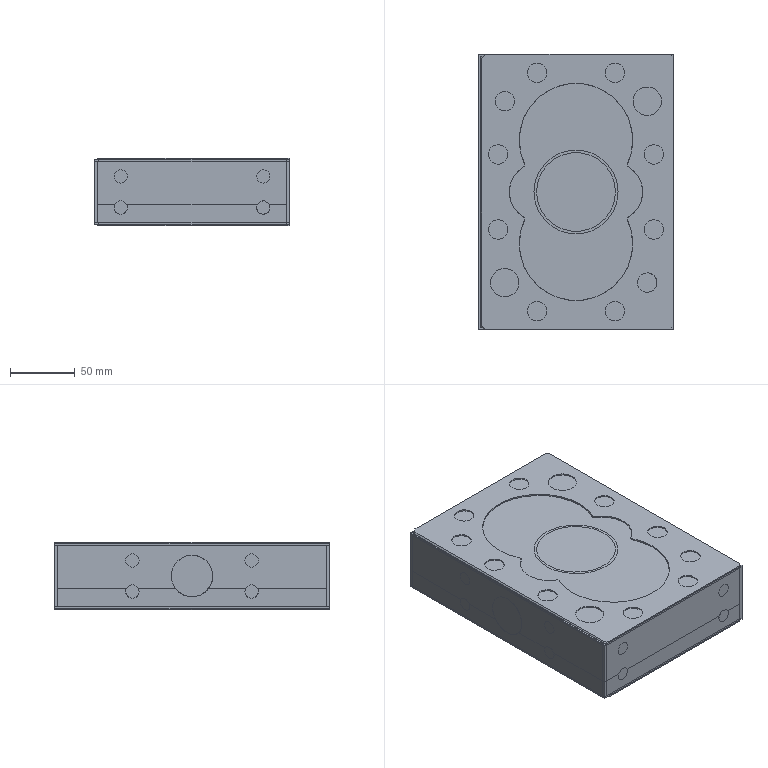NC program | NX | posted with a generic post | part box 150.2 x 212.2 x 52.4 mm
Lines 18 to 851 of 152230:
(PLANAR_PROFILE , TOOL : D45R0.8圆鼻飞刀)
N34 T06 M6
N36 G54
N38 G17 G0 G90 X-44.794 Y20.59 S1061 M3
N40 G43 Z100. H6
N42 Z1.1
N44 G94 G1 X-47.122 Y19.947 Z1.096 F1273.
N46 X-49.964 Y18.69 Z1.09
N48 X-52.591 Y17.031 Z1.085
N50 X-54.947 Y15.006 Z1.08
N52 X-56.982 Y12.658 Z1.074
N54 X-58.651 Y10.037 Z1.069
N56 X-59.918 Y7.201 Z1.063
N58 X-60.758 Y4.209 Z1.058
N60 X-61.15 Y1.127 Z1.052
N62 Y-1.127 Z1.048
N64 X-60.758 Y-4.209 Z1.043
N66 X-59.918 Y-7.201 Z1.038
N68 X-58.651 Y-10.037 Z1.032
N70 X-56.982 Y-12.658 Z1.027
N72 X-54.947 Y-15.006 Z1.021
N74 X-52.591 Y-17.031 Z1.016
N76 X-49.964 Y-18.69 Z1.011
N78 X-47.122 Y-19.947 Z1.005
N80 X-44.127 Y-20.774 Z1.
N82 X-41.043 Y-21.154 Z0.994
N84 X-37.937 Y-21.079 Z0.989
N86 X-34.876 Y-20.551 Z0.983
N88 X-31.924 Y-19.58 Z0.978
N90 X-29.855 Y-18.595 Z0.974
N92 X-27.425 Y-17.746 Z0.969
N94 X-24.914 Y-17.178 Z0.965
N96 X-22.355 Y-16.9 Z0.96
N98 X-18.735 Z0.954
N100 X-15.612 Y-17.28 Z0.949
N102 X-12.572 Y-18.089 Z0.943
N104 X-9.673 Y-19.313 Z0.938
N106 X-6.972 Y-20.926 Z0.932
N108 X-4.521 Y-22.899 Z0.927
N110 X-2.367 Y-25.192 Z0.921
N112 X-0.552 Y-27.762 Z0.916
N114 X0. Y-28.787 Z0.914
N116 X0.552 Y-27.762 Z0.912
N118 X2.367 Y-25.192 Z0.906
N120 X4.521 Y-22.899 Z0.901
N122 X6.972 Y-20.926 Z0.895
N124 X9.673 Y-19.313 Z0.89
N126 X12.572 Y-18.089 Z0.884
N128 X15.612 Y-17.28 Z0.879
N130 X18.735 Y-16.9 Z0.873
N132 X22.355 Z0.867
N134 X24.914 Y-17.178 Z0.862
N136 X27.425 Y-17.746 Z0.858
N138 X29.855 Y-18.595 Z0.853
N140 X31.924 Y-19.58 Z0.849
N142 X34.876 Y-20.551 Z0.844
N144 X37.937 Y-21.079 Z0.839
N146 X41.043 Y-21.154 Z0.833
N148 X44.127 Y-20.774 Z0.828
N150 X47.122 Y-19.947 Z0.822
N152 X49.964 Y-18.69 Z0.817
N154 X52.591 Y-17.031 Z0.811
N156 X54.947 Y-15.006 Z0.806
N158 X56.982 Y-12.658 Z0.801
N160 X58.651 Y-10.037 Z0.795
N162 X59.918 Y-7.201 Z0.79
N164 X60.758 Y-4.209 Z0.784
N166 X61.15 Y-1.127 Z0.779
N168 Y0. Z0.777
N170 Y1.127 Z0.775
N172 X60.758 Y4.209 Z0.77
N174 X59.918 Y7.201 Z0.764
N176 X58.651 Y10.037 Z0.759
N178 X56.982 Y12.658 Z0.753
N180 X54.947 Y15.006 Z0.748
N182 X52.591 Y17.031 Z0.742
N184 X49.964 Y18.69 Z0.737
N186 X47.122 Y19.947 Z0.732
N188 X44.127 Y20.774 Z0.726
N190 X41.043 Y21.154 Z0.721
N192 X37.937 Y21.079 Z0.715
N194 X34.876 Y20.551 Z0.71
N196 X31.924 Y19.58 Z0.705
N198 X29.855 Y18.595 Z0.701
N200 X27.425 Y17.746 Z0.696
N202 X24.914 Y17.178 Z0.692
N204 X22.355 Y16.9 Z0.687
N206 X18.735 Z0.681
N208 X15.612 Y17.28 Z0.675
N210 X12.572 Y18.089 Z0.67
N212 X9.673 Y19.313 Z0.664
N214 X6.972 Y20.926 Z0.659
N216 X4.521 Y22.899 Z0.653
N218 X2.367 Y25.192 Z0.648
N220 X0.552 Y27.762 Z0.642
N222 X0. Y28.787 Z0.64
N224 X-0.552 Y27.762 Z0.638
N226 X-2.367 Y25.192 Z0.633
N228 X-4.521 Y22.899 Z0.627
N230 X-6.972 Y20.926 Z0.622
N232 X-9.673 Y19.313 Z0.616
N234 X-12.572 Y18.089 Z0.611
N236 X-15.612 Y17.28 Z0.605
N238 X-18.735 Y16.9 Z0.6
N240 X-22.355 Z0.593
N242 X-24.914 Y17.178 Z0.589
N244 X-27.425 Y17.746 Z0.584
N246 X-29.855 Y18.595 Z0.58
N248 X-31.924 Y19.58 Z0.576
N250 X-34.876 Y20.551 Z0.571
N252 X-37.937 Y21.079 Z0.565
N254 X-41.043 Y21.154 Z0.56
N256 X-44.127 Y20.774 Z0.554
N258 X-47.122 Y19.947 Z0.549
N260 X-49.964 Y18.69 Z0.543
N262 X-52.591 Y17.031 Z0.538
N264 X-54.947 Y15.006 Z0.533
N266 X-56.982 Y12.658 Z0.527
N268 X-58.651 Y10.037 Z0.522
N270 X-59.918 Y7.201 Z0.516
N272 X-60.758 Y4.209 Z0.511
N274 X-61.15 Y1.127 Z0.505
N276 Y-1.127 Z0.502
N278 X-60.758 Y-4.209 Z0.496
N280 X-59.918 Y-7.201 Z0.491
N282 X-58.651 Y-10.037 Z0.485
N284 X-56.982 Y-12.658 Z0.48
N286 X-54.947 Y-15.006 Z0.474
N288 X-52.591 Y-17.031 Z0.469
N290 X-49.964 Y-18.69 Z0.464
N292 X-47.122 Y-19.947 Z0.458
N294 X-44.127 Y-20.774 Z0.453
N296 X-41.043 Y-21.154 Z0.447
N298 X-37.937 Y-21.079 Z0.442
N300 X-34.876 Y-20.551 Z0.436
N302 X-31.924 Y-19.58 Z0.431
N304 X-29.855 Y-18.595 Z0.427
N306 X-27.425 Y-17.746 Z0.423
N308 X-24.914 Y-17.178 Z0.418
N310 X-22.355 Y-16.9 Z0.414
N312 X-18.735 Z0.407
N314 X-15.612 Y-17.28 Z0.402
N316 X-12.572 Y-18.089 Z0.396
N318 X-9.673 Y-19.313 Z0.391
N320 X-6.972 Y-20.926 Z0.385
N322 X-4.521 Y-22.899 Z0.38
N324 X-2.367 Y-25.192 Z0.374
N326 X-0.552 Y-27.762 Z0.369
N328 X0. Y-28.787 Z0.367
N330 X0.552 Y-27.762 Z0.365
N332 X2.367 Y-25.192 Z0.359
N334 X4.521 Y-22.899 Z0.354
N336 X6.972 Y-20.926 Z0.348
N338 X9.673 Y-19.313 Z0.343
N340 X12.572 Y-18.089 Z0.337
N342 X15.612 Y-17.28 Z0.332
N344 X18.735 Y-16.9 Z0.326
N346 X22.355 Z0.32
N348 X24.914 Y-17.178 Z0.316
N350 X27.425 Y-17.746 Z0.311
N352 X29.855 Y-18.595 Z0.307
N354 X31.924 Y-19.58 Z0.303
N356 X34.876 Y-20.551 Z0.297
N358 X37.937 Y-21.079 Z0.292
N360 X41.043 Y-21.154 Z0.286
N362 X44.127 Y-20.774 Z0.281
N364 X47.122 Y-19.947 Z0.275
N366 X49.964 Y-18.69 Z0.27
N368 X52.591 Y-17.031 Z0.265
N370 X54.947 Y-15.006 Z0.259
N372 X56.982 Y-12.658 Z0.254
N374 X58.651 Y-10.037 Z0.248
N376 X59.918 Y-7.201 Z0.243
N378 X60.758 Y-4.209 Z0.237
N380 X61.15 Y-1.127 Z0.232
N382 Y0. Z0.23
N384 Y1.127 Z0.228
N386 X60.758 Y4.209 Z0.223
N388 X59.918 Y7.201 Z0.217
N390 X58.651 Y10.037 Z0.212
N392 X56.982 Y12.658 Z0.206
N394 X54.947 Y15.006 Z0.201
N396 X52.591 Y17.031 Z0.196
N398 X49.964 Y18.69 Z0.19
N400 X47.122 Y19.947 Z0.185
N402 X44.127 Y20.774 Z0.179
N404 X41.043 Y21.154 Z0.174
N406 X37.937 Y21.079 Z0.168
N408 X34.876 Y20.551 Z0.163
N410 X31.924 Y19.58 Z0.158
N412 X29.855 Y18.595 Z0.154
N414 X27.425 Y17.746 Z0.149
N416 X24.914 Y17.178 Z0.145
N418 X22.355 Y16.9 Z0.14
N420 X18.735 Z0.134
N422 X15.612 Y17.28 Z0.128
N424 X12.572 Y18.089 Z0.123
N426 X9.673 Y19.313 Z0.117
N428 X6.972 Y20.926 Z0.112
N430 X4.521 Y22.899 Z0.106
N432 X2.367 Y25.192 Z0.101
N434 X0.552 Y27.762 Z0.095
N436 X0. Y28.787 Z0.093
N438 X-0.552 Y27.762 Z0.091
N440 X-2.367 Y25.192 Z0.086
N442 X-4.521 Y22.899 Z0.08
N444 X-6.972 Y20.926 Z0.075
N446 X-9.673 Y19.313 Z0.069
N448 X-12.572 Y18.089 Z0.064
N450 X-15.612 Y17.28 Z0.058
N452 X-18.735 Y16.9 Z0.053
N454 X-22.355 Z0.047
N456 X-24.914 Y17.178 Z0.042
N458 X-27.425 Y17.746 Z0.038
N460 X-29.855 Y18.595 Z0.033
N462 X-31.924 Y19.58 Z0.029
N464 X-34.876 Y20.551 Z0.024
N466 X-37.937 Y21.079 Z0.018
N468 X-41.043 Y21.154 Z0.013
N470 X-44.127 Y20.774 Z0.007
N472 X-47.122 Y19.947 Z0.002
N474 X-49.964 Y18.69 Z-0.003
N476 X-52.591 Y17.031 Z-0.009
N478 X-54.947 Y15.006 Z-0.014
N480 X-56.982 Y12.658 Z-0.02
N482 X-58.651 Y10.037 Z-0.025
N484 X-59.918 Y7.201 Z-0.031
N486 X-60.758 Y4.209 Z-0.036
N488 X-61.15 Y1.127 Z-0.041
N490 Y-1.127 Z-0.045
N492 X-60.758 Y-4.209 Z-0.051
N494 X-59.918 Y-7.201 Z-0.056
N496 X-58.651 Y-10.037 Z-0.062
N498 X-56.982 Y-12.658 Z-0.067
N500 X-54.947 Y-15.006 Z-0.072
N502 X-52.591 Y-17.031 Z-0.078
N504 X-49.964 Y-18.69 Z-0.083
N506 X-47.122 Y-19.947 Z-0.089
N508 X-44.127 Y-20.774 Z-0.094
N510 X-41.043 Y-21.154 Z-0.1
N512 X-37.937 Y-21.079 Z-0.105
N514 X-34.876 Y-20.551 Z-0.11
N516 X-31.924 Y-19.58 Z-0.116
N518 X-29.855 Y-18.595 Z-0.12
N520 X-27.425 Y-17.746 Z-0.124
N522 X-24.914 Y-17.178 Z-0.129
N524 X-22.355 Y-16.9 Z-0.133
N526 X-18.735 Z-0.14
N528 X-15.612 Y-17.28 Z-0.145
N530 X-12.572 Y-18.089 Z-0.151
N532 X-9.673 Y-19.313 Z-0.156
N534 X-6.972 Y-20.926 Z-0.162
N536 X-4.521 Y-22.899 Z-0.167
N538 X-2.367 Y-25.192 Z-0.173
N540 X-0.552 Y-27.762 Z-0.178
N542 X0. Y-28.787 Z-0.18
N544 X0.552 Y-27.762 Z-0.182
N546 X2.367 Y-25.192 Z-0.188
N548 X4.521 Y-22.899 Z-0.193
N550 X6.972 Y-20.926 Z-0.199
N552 X9.673 Y-19.313 Z-0.204
N554 X12.572 Y-18.089 Z-0.21
N556 X15.612 Y-17.28 Z-0.215
N558 X18.735 Y-16.9 Z-0.221
N560 X22.355 Z-0.227
N562 X24.914 Y-17.178 Z-0.231
N564 X27.425 Y-17.746 Z-0.236
N566 X29.855 Y-18.595 Z-0.24
N568 X31.924 Y-19.58 Z-0.244
N570 X34.876 Y-20.551 Z-0.25
N572 X37.937 Y-21.079 Z-0.255
N574 X41.043 Y-21.154 Z-0.261
N576 X44.127 Y-20.774 Z-0.266
N578 X47.122 Y-19.947 Z-0.272
N580 X49.964 Y-18.69 Z-0.277
N582 X52.591 Y-17.031 Z-0.282
N584 X54.947 Y-15.006 Z-0.288
N586 X56.982 Y-12.658 Z-0.293
N588 X58.651 Y-10.037 Z-0.299
N590 X59.918 Y-7.201 Z-0.304
N592 X60.758 Y-4.209 Z-0.309
N594 X61.15 Y-1.127 Z-0.315
N596 Y0. Z-0.317
N598 Y1.127 Z-0.319
N600 X60.758 Y4.209 Z-0.324
N602 X59.918 Y7.201 Z-0.33
N604 X58.651 Y10.037 Z-0.335
N606 X56.982 Y12.658 Z-0.341
N608 X54.947 Y15.006 Z-0.346
N610 X52.591 Y17.031 Z-0.351
N612 X49.964 Y18.69 Z-0.357
N614 X47.122 Y19.947 Z-0.362
N616 X44.127 Y20.774 Z-0.368
N618 X41.043 Y21.154 Z-0.373
N620 X37.937 Y21.079 Z-0.378
N622 X34.876 Y20.551 Z-0.384
N624 X31.924 Y19.58 Z-0.389
N626 X29.855 Y18.595 Z-0.393
N628 X27.425 Y17.746 Z-0.398
N630 X24.914 Y17.178 Z-0.402
N632 X22.355 Y16.9 Z-0.407
N634 X18.735 Z-0.413
N636 X15.612 Y17.28 Z-0.419
N638 X12.572 Y18.089 Z-0.424
N640 X9.673 Y19.313 Z-0.43
N642 X6.972 Y20.926 Z-0.435
N644 X4.521 Y22.899 Z-0.441
N646 X2.367 Y25.192 Z-0.446
N648 X0.552 Y27.762 Z-0.452
N650 X0. Y28.787 Z-0.454
N652 X-0.552 Y27.762 Z-0.456
N654 X-2.367 Y25.192 Z-0.461
N656 X-4.521 Y22.899 Z-0.467
N658 X-6.972 Y20.926 Z-0.472
N660 X-9.673 Y19.313 Z-0.478
N662 X-12.572 Y18.089 Z-0.483
N664 X-15.612 Y17.28 Z-0.489
N666 X-18.735 Y16.9 Z-0.494
N668 X-22.355 Z-0.5
N670 X-24.914 Y17.178 Z-0.505
N672 X-27.425 Y17.746 Z-0.509
N674 X-29.855 Y18.595 Z-0.514
N676 X-31.924 Y19.58 Z-0.518
N678 X-34.876 Y20.551 Z-0.523
N680 X-37.937 Y21.079 Z-0.529
N682 X-41.043 Y21.154 Z-0.534
N684 X-44.127 Y20.774 Z-0.54
N686 X-47.122 Y19.947 Z-0.545
N688 X-49.964 Y18.69 Z-0.55
N690 X-52.591 Y17.031 Z-0.556
N692 X-54.947 Y15.006 Z-0.561
N694 X-56.982 Y12.658 Z-0.567
N696 X-58.651 Y10.037 Z-0.572
N698 X-59.918 Y7.201 Z-0.578
N700 X-60.758 Y4.209 Z-0.583
N702 X-61.15 Y1.127 Z-0.588
N704 Y-1.127 Z-0.592
N706 X-60.758 Y-4.209 Z-0.598
N708 X-59.918 Y-7.201 Z-0.603
N710 X-58.651 Y-10.037 Z-0.609
N712 X-56.982 Y-12.658 Z-0.614
N714 X-54.947 Y-15.006 Z-0.619
N716 X-52.591 Y-17.031 Z-0.625
N718 X-49.964 Y-18.69 Z-0.63
N720 X-47.122 Y-19.947 Z-0.636
N722 X-44.127 Y-20.774 Z-0.641
N724 X-41.043 Y-21.154 Z-0.647
N726 X-37.937 Y-21.079 Z-0.652
N728 X-34.876 Y-20.551 Z-0.657
N730 X-31.924 Y-19.58 Z-0.663
N732 X-29.855 Y-18.595 Z-0.667
N734 X-27.425 Y-17.746 Z-0.671
N736 X-24.914 Y-17.178 Z-0.676
N738 X-22.355 Y-16.9 Z-0.68
N740 X-18.735 Z-0.687
N742 X-15.612 Y-17.28 Z-0.692
N744 X-12.572 Y-18.089 Z-0.698
N746 X-9.673 Y-19.313 Z-0.703
N748 X-6.972 Y-20.926 Z-0.709
N750 X-4.521 Y-22.899 Z-0.714
N752 X-2.367 Y-25.192 Z-0.72
N754 X-0.552 Y-27.762 Z-0.725
N756 X0. Y-28.787 Z-0.727
N758 X0.552 Y-27.762 Z-0.729
N760 X2.367 Y-25.192 Z-0.735
N762 X4.521 Y-22.899 Z-0.74
N764 X6.972 Y-20.926 Z-0.746
N766 X9.673 Y-19.313 Z-0.751
N768 X12.572 Y-18.089 Z-0.757
N770 X15.612 Y-17.28 Z-0.762
N772 X18.735 Y-16.9 Z-0.768
N774 X22.355 Z-0.774
N776 X24.914 Y-17.178 Z-0.778
N778 X27.425 Y-17.746 Z-0.783
N780 X29.855 Y-18.595 Z-0.787
N782 X31.924 Y-19.58 Z-0.791
N784 X34.876 Y-20.551 Z-0.797
N786 X37.937 Y-21.079 Z-0.802
N788 X41.043 Y-21.154 Z-0.808
N790 X44.127 Y-20.774 Z-0.813
N792 X47.122 Y-19.947 Z-0.818
N794 X49.964 Y-18.69 Z-0.824
N796 X52.591 Y-17.031 Z-0.829
N798 X54.947 Y-15.006 Z-0.835
N800 X56.982 Y-12.658 Z-0.84
N802 X58.651 Y-10.037 Z-0.846
N804 X59.918 Y-7.201 Z-0.851
N806 X60.758 Y-4.209 Z-0.856
N808 X61.15 Y-1.127 Z-0.862
N810 Y0. Z-0.864
N812 Y1.127 Z-0.866
N814 X60.758 Y4.209 Z-0.871
N816 X59.918 Y7.201 Z-0.877
N818 X58.651 Y10.037 Z-0.882
N820 X56.982 Y12.658 Z-0.887
N822 X54.947 Y15.006 Z-0.893
N824 X52.591 Y17.031 Z-0.898
N826 X49.964 Y18.69 Z-0.904
N828 X47.122 Y19.947 Z-0.909
N830 X44.127 Y20.774 Z-0.915
N832 X41.043 Y21.154 Z-0.92
N834 X37.937 Y21.079 Z-0.925
N836 X34.876 Y20.551 Z-0.931
N838 X31.924 Y19.58 Z-0.936
N840 X29.855 Y18.595 Z-0.94
N842 X27.425 Y17.746 Z-0.945
N844 X24.914 Y17.178 Z-0.949
N846 X22.355 Y16.9 Z-0.954
N848 X18.735 Z-0.96
N850 X15.612 Y17.28 Z-0.966
N852 X12.572 Y18.089 Z-0.971
N854 X9.673 Y19.313 Z-0.977
N856 X6.972 Y20.926 Z-0.982
N858 X4.521 Y22.899 Z-0.987
N860 X2.367 Y25.192 Z-0.993
N862 X0.552 Y27.762 Z-0.998
N864 X0. Y28.787 Z-1.001
N866 X-0.552 Y27.762 Z-1.003
N868 X-2.367 Y25.192 Z-1.008
N870 X-4.521 Y22.899 Z-1.014
N872 X-6.972 Y20.926 Z-1.019
N874 X-9.673 Y19.313 Z-1.025
N876 X-12.572 Y18.089 Z-1.03
N878 X-15.612 Y17.28 Z-1.035
N880 X-18.735 Y16.9 Z-1.041
N882 X-22.355 Z-1.047
N884 X-24.914 Y17.178 Z-1.052
N886 X-27.425 Y17.746 Z-1.056
N888 X-29.855 Y18.595 Z-1.061
N890 X-31.924 Y19.58 Z-1.065
N892 X-34.876 Y20.551 Z-1.07
N894 X-37.937 Y21.079 Z-1.076
N896 X-41.043 Y21.154 Z-1.081
N898 X-44.127 Y20.774 Z-1.086
N900 X-47.122 Y19.947 Z-1.092
N902 X-49.964 Y18.69 Z-1.097
N904 X-52.591 Y17.031 Z-1.103
N906 X-54.947 Y15.006 Z-1.108
N908 X-56.982 Y12.658 Z-1.114
N910 X-58.651 Y10.037 Z-1.119
N912 X-59.918 Y7.201 Z-1.124
N914 X-60.758 Y4.209 Z-1.13
N916 X-61.15 Y1.127 Z-1.135
N918 Y-1.127 Z-1.139
N920 X-60.758 Y-4.209 Z-1.145
N922 X-59.918 Y-7.201 Z-1.15
N924 X-58.651 Y-10.037 Z-1.155
N926 X-56.982 Y-12.658 Z-1.161
N928 X-54.947 Y-15.006 Z-1.166
N930 X-52.591 Y-17.031 Z-1.172
N932 X-49.964 Y-18.69 Z-1.177
N934 X-47.122 Y-19.947 Z-1.183
N936 X-44.127 Y-20.774 Z-1.188
N938 X-41.043 Y-21.154 Z-1.193
N940 X-37.937 Y-21.079 Z-1.199
N942 X-34.876 Y-20.551 Z-1.204
N944 X-31.924 Y-19.58 Z-1.21
N946 X-29.855 Y-18.595 Z-1.214
N948 X-27.425 Y-17.746 Z-1.218
N950 X-24.914 Y-17.178 Z-1.223
N952 X-22.355 Y-16.9 Z-1.227
N954 X-18.735 Z-1.234
N956 X-15.612 Y-17.28 Z-1.239
N958 X-12.572 Y-18.089 Z-1.244
N960 X-9.673 Y-19.313 Z-1.25
N962 X-6.972 Y-20.926 Z-1.255
N964 X-4.521 Y-22.899 Z-1.261
N966 X-2.367 Y-25.192 Z-1.266
N968 X-0.552 Y-27.762 Z-1.272
N970 X0. Y-28.787 Z-1.274
N972 X0.552 Y-27.762 Z-1.276
N974 X2.367 Y-25.192 Z-1.281
N976 X4.521 Y-22.899 Z-1.287
N978 X6.972 Y-20.926 Z-1.292
N980 X9.673 Y-19.313 Z-1.298
N982 X12.572 Y-18.089 Z-1.303
N984 X15.612 Y-17.28 Z-1.309
N986 X18.735 Y-16.9 Z-1.314
N988 X22.355 Z-1.321
N990 X24.914 Y-17.178 Z-1.325
N992 X27.425 Y-17.746 Z-1.33
N994 X29.855 Y-18.595 Z-1.334
N996 X31.924 Y-19.58 Z-1.338
N998 X34.876 Y-20.551 Z-1.344
N1000 X37.937 Y-21.079 Z-1.349
N1002 X41.043 Y-21.154 Z-1.355
N1004 X44.127 Y-20.774 Z-1.36
N1006 X47.122 Y-19.947 Z-1.365
N1008 X49.964 Y-18.69 Z-1.371
N1010 X52.591 Y-17.031 Z-1.376
N1012 X54.947 Y-15.006 Z-1.382
N1014 X56.982 Y-12.658 Z-1.387
N1016 X58.651 Y-10.037 Z-1.392
N1018 X59.918 Y-7.201 Z-1.398
N1020 X60.758 Y-4.209 Z-1.403
N1022 X61.15 Y-1.127 Z-1.409
N1024 Y0. Z-1.411
N1026 Y1.127 Z-1.413
N1028 X60.758 Y4.209 Z-1.418
N1030 X59.918 Y7.201 Z-1.424
N1032 X58.651 Y10.037 Z-1.429
N1034 X56.982 Y12.658 Z-1.434
N1036 X54.947 Y15.006 Z-1.44
N1038 X52.591 Y17.031 Z-1.445
N1040 X49.964 Y18.69 Z-1.451
N1042 X47.122 Y19.947 Z-1.456
N1044 X44.127 Y20.774 Z-1.461
N1046 X41.043 Y21.154 Z-1.467
N1048 X37.937 Y21.079 Z-1.472
N1050 X34.876 Y20.551 Z-1.478
N1052 X31.924 Y19.58 Z-1.483
N1054 X29.855 Y18.595 Z-1.487
N1056 X27.425 Y17.746 Z-1.492
N1058 X24.914 Y17.178 Z-1.496
N1060 X22.355 Y16.9 Z-1.501
N1062 X18.735 Z-1.507
N1064 X15.612 Y17.28 Z-1.512
N1066 X12.572 Y18.089 Z-1.518
N1068 X9.673 Y19.313 Z-1.523
N1070 X6.972 Y20.926 Z-1.529
N1072 X4.521 Y22.899 Z-1.534
N1074 X2.367 Y25.192 Z-1.54
N1076 X0.552 Y27.762 Z-1.545
N1078 X0. Y28.787 Z-1.547
N1080 X-0.552 Y27.762 Z-1.549
N1082 X-2.367 Y25.192 Z-1.555
N1084 X-4.521 Y22.899 Z-1.56
N1086 X-6.972 Y20.926 Z-1.566
N1088 X-9.673 Y19.313 Z-1.571
N1090 X-12.572 Y18.089 Z-1.577
N1092 X-15.612 Y17.28 Z-1.582
N1094 X-18.735 Y16.9 Z-1.588
N1096 X-22.355 Z-1.594
N1098 X-24.914 Y17.178 Z-1.599
N1100 X-27.425 Y17.746 Z-1.603
N1102 X-29.855 Y18.595 Z-1.608
N1104 X-31.924 Y19.58 Z-1.612
N1106 X-34.876 Y20.551 Z-1.617
N1108 X-37.937 Y21.079 Z-1.623
N1110 X-41.043 Y21.154 Z-1.628
N1112 X-44.127 Y20.774 Z-1.633
N1114 X-47.122 Y19.947 Z-1.639
N1116 X-49.964 Y18.69 Z-1.644
N1118 X-52.591 Y17.031 Z-1.65
N1120 X-54.947 Y15.006 Z-1.655
N1122 X-56.982 Y12.658 Z-1.661
N1124 X-58.651 Y10.037 Z-1.666
N1126 X-59.918 Y7.201 Z-1.671
N1128 X-60.758 Y4.209 Z-1.677
N1130 X-61.15 Y1.127 Z-1.682
N1132 Y-1.127 Z-1.686
N1134 X-60.758 Y-4.209 Z-1.692
N1136 X-59.918 Y-7.201 Z-1.697
N1138 X-58.651 Y-10.037 Z-1.702
N1140 X-56.982 Y-12.658 Z-1.708
N1142 X-54.947 Y-15.006 Z-1.713
N1144 X-52.591 Y-17.031 Z-1.719
N1146 X-49.964 Y-18.69 Z-1.724
N1148 X-47.122 Y-19.947 Z-1.73
N1150 X-44.127 Y-20.774 Z-1.735
N1152 X-41.043 Y-21.154 Z-1.74
N1154 X-37.937 Y-21.079 Z-1.746
N1156 X-34.876 Y-20.551 Z-1.751
N1158 X-31.924 Y-19.58 Z-1.757
N1160 X-29.855 Y-18.595 Z-1.761
N1162 X-27.425 Y-17.746 Z-1.765
N1164 X-24.914 Y-17.178 Z-1.77
N1166 X-22.355 Y-16.9 Z-1.774
N1168 X-18.735 Z-1.78
N1170 X-15.612 Y-17.28 Z-1.786
N1172 X-12.572 Y-18.089 Z-1.791
N1174 X-9.673 Y-19.313 Z-1.797
N1176 X-6.972 Y-20.926 Z-1.802
N1178 X-4.521 Y-22.899 Z-1.808
N1180 X-2.367 Y-25.192 Z-1.813
N1182 X-0.552 Y-27.762 Z-1.819
N1184 X0. Y-28.787 Z-1.821
N1186 X0.552 Y-27.762 Z-1.823
N1188 X2.367 Y-25.192 Z-1.828
N1190 X4.521 Y-22.899 Z-1.834
N1192 X6.972 Y-20.926 Z-1.839
N1194 X9.673 Y-19.313 Z-1.845
N1196 X12.572 Y-18.089 Z-1.85
N1198 X15.612 Y-17.28 Z-1.856
N1200 X18.735 Y-16.9 Z-1.861
N1202 X22.355 Z-1.868
N1204 X24.914 Y-17.178 Z-1.872
N1206 X27.425 Y-17.746 Z-1.877
N1208 X29.855 Y-18.595 Z-1.881
N1210 X31.924 Y-19.58 Z-1.885
N1212 X34.876 Y-20.551 Z-1.891
N1214 X37.937 Y-21.079 Z-1.896
N1216 X41.043 Y-21.154 Z-1.901
N1218 X44.127 Y-20.774 Z-1.907
N1220 X47.122 Y-19.947 Z-1.912
N1222 X49.964 Y-18.69 Z-1.918
N1224 X52.591 Y-17.031 Z-1.923
N1226 X54.947 Y-15.006 Z-1.929
N1228 X56.982 Y-12.658 Z-1.934
N1230 X58.651 Y-10.037 Z-1.939
N1232 X59.918 Y-7.201 Z-1.945
N1234 X60.758 Y-4.209 Z-1.95
N1236 X61.15 Y-1.127 Z-1.956
N1238 Y0. Z-1.958
N1240 Y1.127 Z-1.96
N1242 X60.758 Y4.209 Z-1.965
N1244 X59.918 Y7.201 Z-1.97
N1246 X58.651 Y10.037 Z-1.976
N1248 X56.982 Y12.658 Z-1.981
N1250 X54.947 Y15.006 Z-1.987
N1252 X52.591 Y17.031 Z-1.992
N1254 X49.964 Y18.69 Z-1.998
N1256 X47.122 Y19.947 Z-2.003
N1258 X44.127 Y20.774 Z-2.008
N1260 X41.043 Y21.154 Z-2.014
N1262 X37.937 Y21.079 Z-2.019
N1264 X34.876 Y20.551 Z-2.025
N1266 X31.924 Y19.58 Z-2.03
N1268 X29.855 Y18.595 Z-2.034
N1270 X27.425 Y17.746 Z-2.039
N1272 X24.914 Y17.178 Z-2.043
N1274 X22.355 Y16.9 Z-2.048
N1276 X18.735 Z-2.054
N1278 X15.612 Y17.28 Z-2.059
N1280 X12.572 Y18.089 Z-2.065
N1282 X9.673 Y19.313 Z-2.07
N1284 X6.972 Y20.926 Z-2.076
N1286 X4.521 Y22.899 Z-2.081
N1288 X2.367 Y25.192 Z-2.087
N1290 X0.552 Y27.762 Z-2.092
N1292 X0. Y28.787 Z-2.094
N1294 X-0.552 Y27.762 Z-2.096
N1296 X-2.367 Y25.192 Z-2.102
N1298 X-4.521 Y22.899 Z-2.107
N1300 X-6.972 Y20.926 Z-2.113
N1302 X-9.673 Y19.313 Z-2.118
N1304 X-12.572 Y18.089 Z-2.124
N1306 X-15.612 Y17.28 Z-2.129
N1308 X-18.735 Y16.9 Z-2.135
N1310 X-22.355 Z-2.141
N1312 X-24.914 Y17.178 Z-2.146
N1314 X-27.425 Y17.746 Z-2.15
N1316 X-29.855 Y18.595 Z-2.155
N1318 X-31.924 Y19.58 Z-2.159
N1320 X-34.876 Y20.551 Z-2.164
N1322 X-37.937 Y21.079 Z-2.169
N1324 X-41.043 Y21.154 Z-2.175
N1326 X-44.127 Y20.774 Z-2.18
N1328 X-47.122 Y19.947 Z-2.186
N1330 X-49.964 Y18.69 Z-2.191
N1332 X-52.591 Y17.031 Z-2.197
N1334 X-54.947 Y15.006 Z-2.202
N1336 X-56.982 Y12.658 Z-2.207
N1338 X-58.651 Y10.037 Z-2.213
N1340 X-59.918 Y7.201 Z-2.218
N1342 X-60.758 Y4.209 Z-2.224
N1344 X-61.15 Y1.127 Z-2.229
N1346 Y-1.127 Z-2.233
N1348 X-60.758 Y-4.209 Z-2.238
N1350 X-59.918 Y-7.201 Z-2.244
N1352 X-58.651 Y-10.037 Z-2.249
N1354 X-56.982 Y-12.658 Z-2.255
N1356 X-54.947 Y-15.006 Z-2.26
N1358 X-52.591 Y-17.031 Z-2.266
N1360 X-49.964 Y-18.69 Z-2.271
N1362 X-47.122 Y-19.947 Z-2.276
N1364 X-44.127 Y-20.774 Z-2.282
N1366 X-41.043 Y-21.154 Z-2.287
N1368 X-37.937 Y-21.079 Z-2.293
N1370 X-34.876 Y-20.551 Z-2.298
N1372 X-31.924 Y-19.58 Z-2.304
N1374 X-29.855 Y-18.595 Z-2.308
N1376 X-27.425 Y-17.746 Z-2.312
N1378 X-24.914 Y-17.178 Z-2.317
N1380 X-22.355 Y-16.9 Z-2.321
N1382 X-18.735 Z-2.327
N1384 X-15.612 Y-17.28 Z-2.333
N1386 X-12.572 Y-18.089 Z-2.338
N1388 X-9.673 Y-19.313 Z-2.344
N1390 X-6.972 Y-20.926 Z-2.349
N1392 X-4.521 Y-22.899 Z-2.355
N1394 X-2.367 Y-25.192 Z-2.36
N1396 X-0.552 Y-27.762 Z-2.366
N1398 X0. Y-28.787 Z-2.368
N1400 X0.552 Y-27.762 Z-2.37
N1402 X2.367 Y-25.192 Z-2.375
N1404 X4.521 Y-22.899 Z-2.381
N1406 X6.972 Y-20.926 Z-2.386
N1408 X9.673 Y-19.313 Z-2.392
N1410 X12.572 Y-18.089 Z-2.397
N1412 X15.612 Y-17.28 Z-2.403
N1414 X18.735 Y-16.9 Z-2.408
N1416 X22.355 Z-2.415
N1418 X24.914 Y-17.178 Z-2.419
N1420 X27.425 Y-17.746 Z-2.424
N1422 X29.855 Y-18.595 Z-2.428
N1424 X31.924 Y-19.58 Z-2.432
N1426 X34.876 Y-20.551 Z-2.438
N1428 X37.937 Y-21.079 Z-2.443
N1430 X41.043 Y-21.154 Z-2.448
N1432 X44.127 Y-20.774 Z-2.454
N1434 X47.122 Y-19.947 Z-2.459
N1436 X49.964 Y-18.69 Z-2.465
N1438 X52.591 Y-17.031 Z-2.47
N1440 X54.947 Y-15.006 Z-2.475
N1442 X56.982 Y-12.658 Z-2.481
N1444 X58.651 Y-10.037 Z-2.486
N1446 X59.918 Y-7.201 Z-2.492
N1448 X60.758 Y-4.209 Z-2.497
N1450 X61.15 Y-1.127 Z-2.503
N1452 Y0. Z-2.505
N1454 Y1.127 Z-2.507
N1456 X60.758 Y4.209 Z-2.512
N1458 X59.918 Y7.201 Z-2.517
N1460 X58.651 Y10.037 Z-2.523
N1462 X56.982 Y12.658 Z-2.528
N1464 X54.947 Y15.006 Z-2.534
N1466 X52.591 Y17.031 Z-2.539
N1468 X49.964 Y18.69 Z-2.544
N1470 X47.122 Y19.947 Z-2.55
N1472 X44.127 Y20.774 Z-2.555
N1474 X41.043 Y21.154 Z-2.561
N1476 X37.937 Y21.079 Z-2.566
N1478 X34.876 Y20.551 Z-2.572
N1480 X31.924 Y19.58 Z-2.577
N1482 X29.855 Y18.595 Z-2.581
N1484 X27.425 Y17.746 Z-2.585
N1486 X24.914 Y17.178 Z-2.59
N1488 X22.355 Y16.9 Z-2.594
N1490 X18.735 Z-2.601
N1492 X15.612 Y17.28 Z-2.606
N1494 X12.572 Y18.089 Z-2.612
N1496 X9.673 Y19.313 Z-2.617
N1498 X6.972 Y20.926 Z-2.623
N1500 X4.521 Y22.899 Z-2.628
N1502 X2.367 Y25.192 Z-2.634
N1504 X0.552 Y27.762 Z-2.639
N1506 X0. Y28.787 Z-2.641
N1508 X-0.552 Y27.762 Z-2.643
N1510 X-2.367 Y25.192 Z-2.649
N1512 X-4.521 Y22.899 Z-2.654
N1514 X-6.972 Y20.926 Z-2.66
N1516 X-9.673 Y19.313 Z-2.665
N1518 X-12.572 Y18.089 Z-2.671
N1520 X-15.612 Y17.28 Z-2.676
N1522 X-18.735 Y16.9 Z-2.682
N1524 X-22.355 Z-2.688
N1526 X-24.914 Y17.178 Z-2.693
N1528 X-27.425 Y17.746 Z-2.697
N1530 X-29.855 Y18.595 Z-2.702
N1532 X-31.924 Y19.58 Z-2.706
N1534 X-34.876 Y20.551 Z-2.711
N1536 X-37.937 Y21.079 Z-2.716
N1538 X-41.043 Y21.154 Z-2.722
N1540 X-44.127 Y20.774 Z-2.727
N1542 X-47.122 Y19.947 Z-2.733
N1544 X-49.964 Y18.69 Z-2.738
N1546 X-52.591 Y17.031 Z-2.743
N1548 X-54.947 Y15.006 Z-2.749
N1550 X-56.982 Y12.658 Z-2.754
N1552 X-58.651 Y10.037 Z-2.76
N1554 X-59.918 Y7.201 Z-2.765
N1556 X-60.758 Y4.209 Z-2.771
N1558 X-61.15 Y1.127 Z-2.776
N1560 Y-1.127 Z-2.78
N1562 X-60.758 Y-4.209 Z-2.785
N1564 X-59.918 Y-7.201 Z-2.791
N1566 X-58.651 Y-10.037 Z-2.796
N1568 X-56.982 Y-12.658 Z-2.802
N1570 X-54.947 Y-15.006 Z-2.807
N1572 X-52.591 Y-17.031 Z-2.813
N1574 X-49.964 Y-18.69 Z-2.818
N1576 X-47.122 Y-19.947 Z-2.823
N1578 X-44.127 Y-20.774 Z-2.829
N1580 X-41.043 Y-21.154 Z-2.834
N1582 X-37.937 Y-21.079 Z-2.84
N1584 X-34.876 Y-20.551 Z-2.845
N1586 X-31.924 Y-19.58 Z-2.85
N1588 X-29.855 Y-18.595 Z-2.854
N1590 X-27.425 Y-17.746 Z-2.859
N1592 X-24.914 Y-17.178 Z-2.863
N1594 X-22.355 Y-16.9 Z-2.868
N1596 X-18.735 Z-2.874
N1598 X-15.612 Y-17.28 Z-2.88
N1600 X-12.572 Y-18.089 Z-2.885
N1602 X-9.673 Y-19.313 Z-2.891
N1604 X-6.972 Y-20.926 Z-2.896
N1606 X-4.521 Y-22.899 Z-2.902
N1608 X-2.367 Y-25.192 Z-2.907
N1610 X-0.552 Y-27.762 Z-2.913
N1612 X0. Y-28.787 Z-2.915
N1614 X0.552 Y-27.762 Z-2.917
N1616 X2.367 Y-25.192 Z-2.922
N1618 X4.521 Y-22.899 Z-2.928
N1620 X6.972 Y-20.926 Z-2.933
N1622 X9.673 Y-19.313 Z-2.939
N1624 X12.572 Y-18.089 Z-2.944
N1626 X15.612 Y-17.28 Z-2.95
N1628 X18.735 Y-16.9 Z-2.955
N1630 X22.355 Z-2.962
N1632 X24.914 Y-17.178 Z-2.966
N1634 X27.425 Y-17.746 Z-2.971
N1636 X29.855 Y-18.595 Z-2.975
N1638 X31.924 Y-19.58 Z-2.979
N1640 X34.876 Y-20.551 Z-2.984
N1642 X37.937 Y-21.079 Z-2.99
N1644 X41.043 Y-21.154 Z-2.995
N1646 X44.127 Y-20.774 Z-3.001
N1648 X47.122 Y-19.947 Z-3.006
N1650 X49.964 Y-18.69 Z-3.012
N1652 X52.591 Y-17.031 Z-3.017
N1654 X54.947 Y-15.006 Z-3.022
N1656 X56.982 Y-12.658 Z-3.028
N1658 X58.651 Y-10.037 Z-3.033
N1660 X59.918 Y-7.201 Z-3.039
N1662 X60.758 Y-4.209 Z-3.044
N1664 X61.15 Y-1.127 Z-3.049
N1666 Y0. Z-3.051
N1668 Y1.127 Z-3.053
N1670 X60.758 Y4.209 Z-3.059
N1672 X59.918 Y7.201 Z-3.064
N1674 X58.651 Y10.037 Z-3.07
N1676 X56.982 Y12.658 Z-3.075
N1678 X54.947 Y15.006 Z-3.081
N1680 X52.591 Y17.031 Z-3.086
N1682 X49.964 Y18.69 Z-3.091
N1684 X47.122 Y19.947 Z-3.097
N1686 X44.127 Y20.774 Z-3.102
N1688 X41.043 Y21.154 Z-3.108
N1690 X37.937 Y21.079 Z-3.113
N1692 X34.876 Y20.551 Z-3.119
N1694 X31.924 Y19.58 Z-3.124